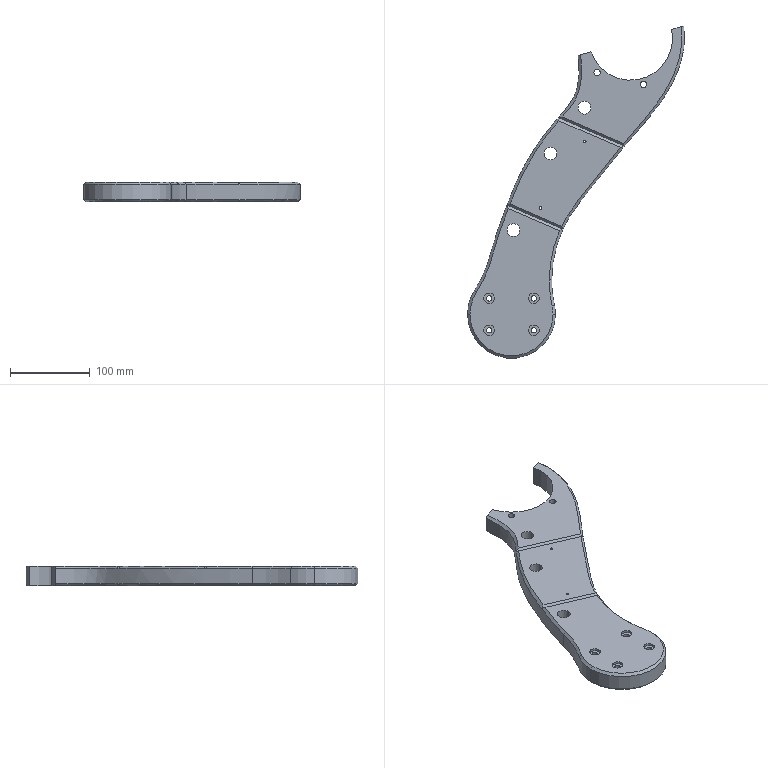Part | SolidWorks | features MirrorStock 1 | 1 solid | 94 faces | box 271.568 x 416.057 x 25 mm | volume 864858 mm3 | cylinder 45 | plane 24 | cone 13 | spline 12 | commonest cylinder face diameters 13.4 x16 6.6 x8 16 x6 3.3 x4 8 x4 110 x3